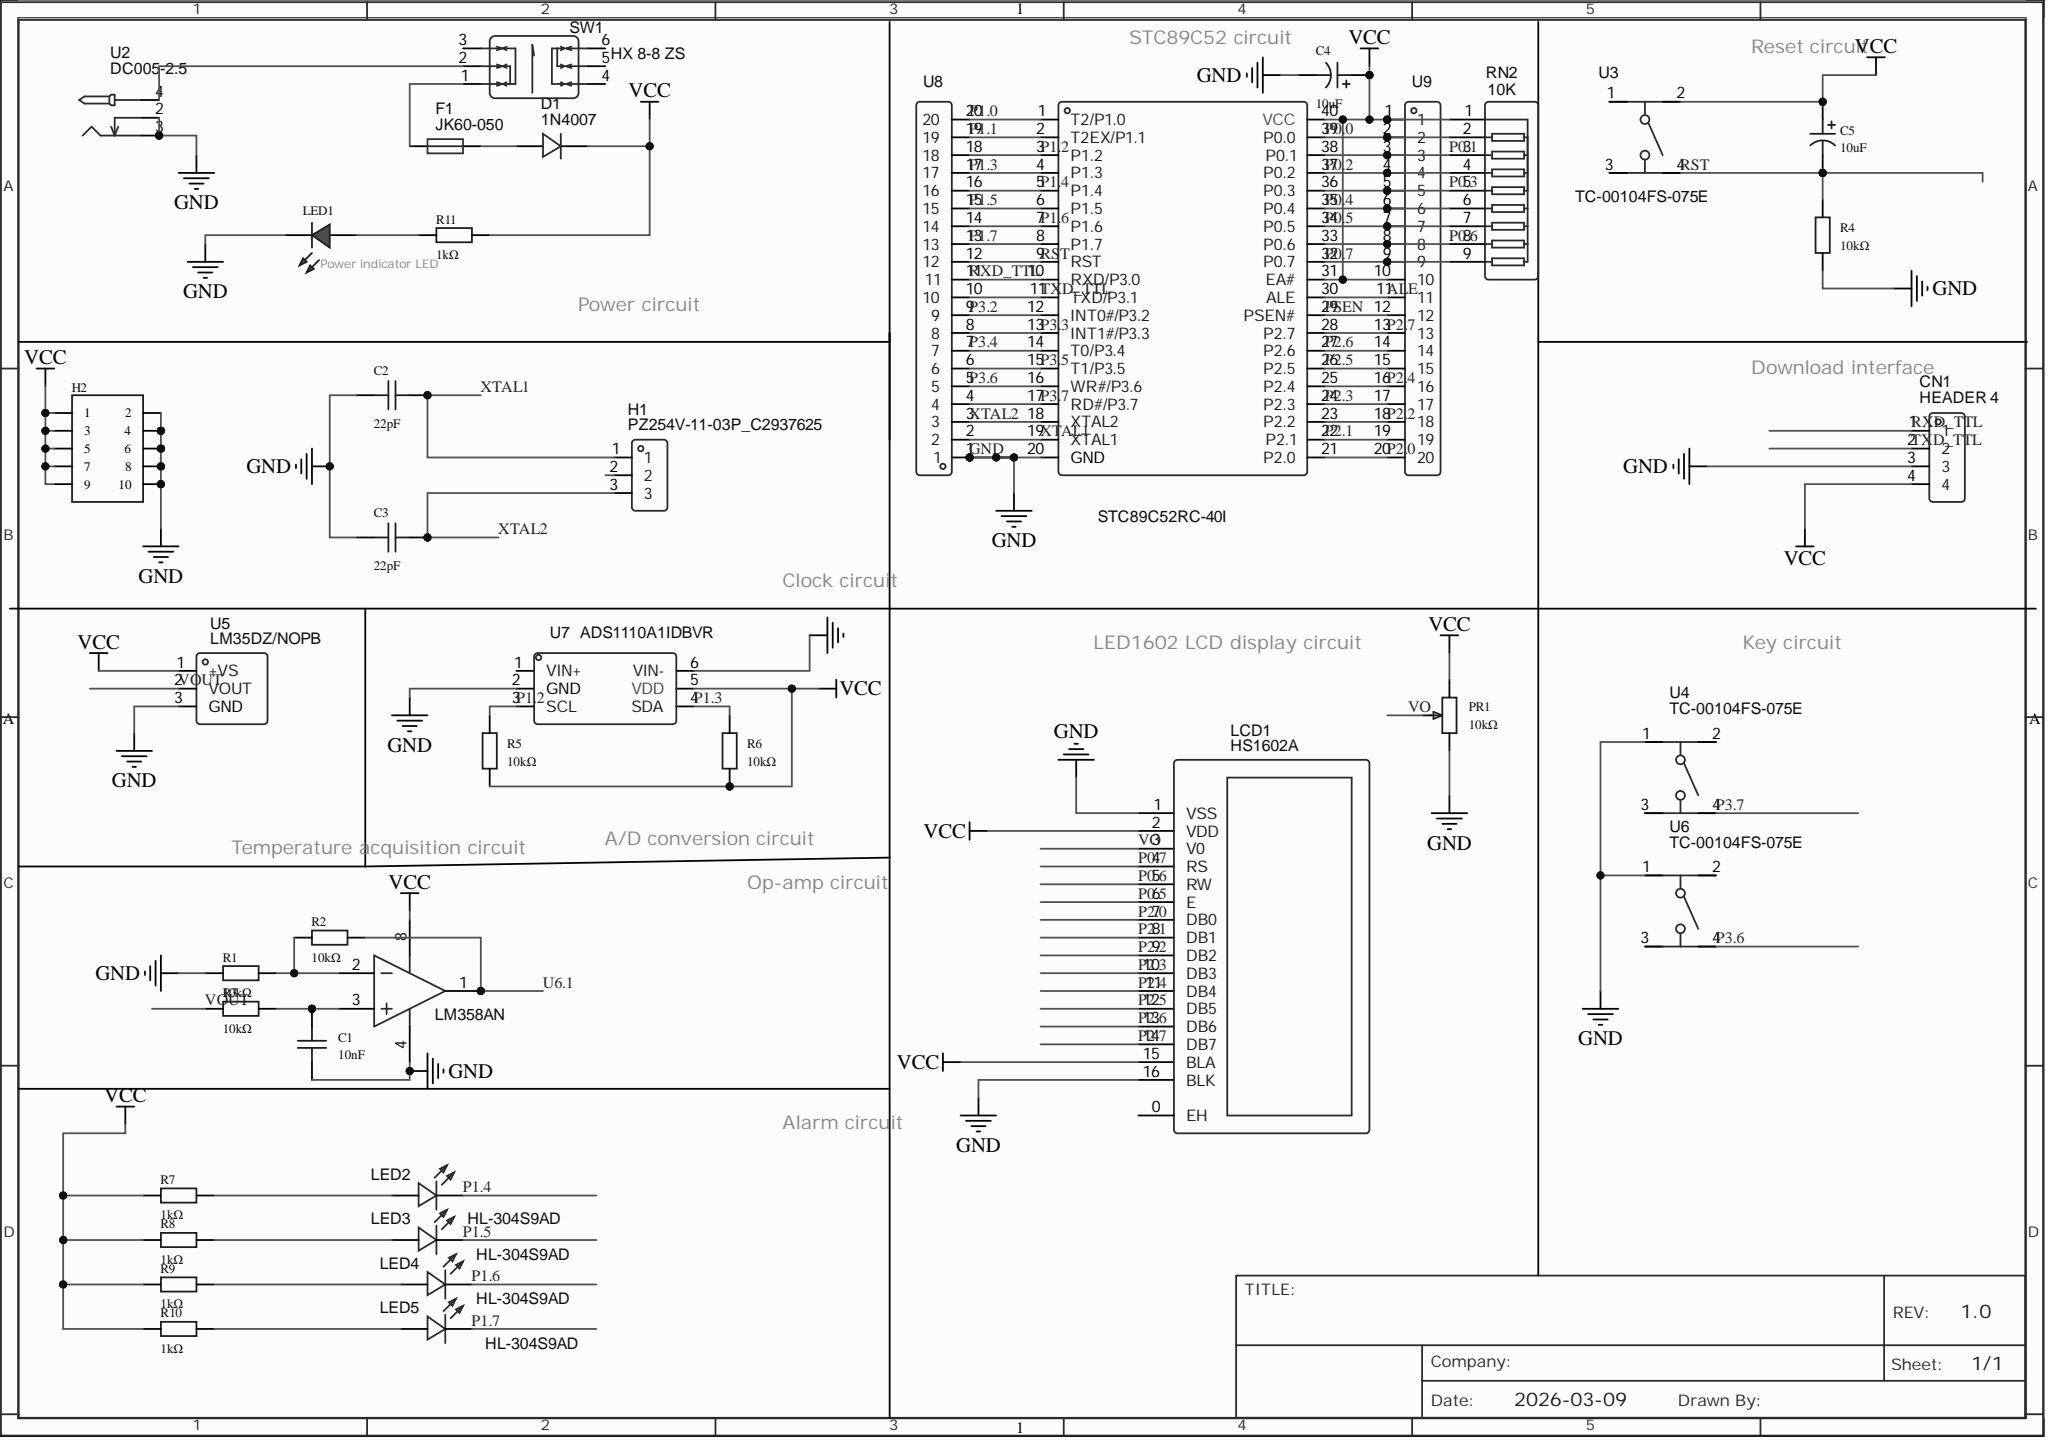Circuit board | Altium Designer | 40 parts | 52 nets
Bill of materials:
Comment,Description,Designator,Footprint,LibRef,Quantity
"10nF","容值:10nF;精度:±5%;额定电压:50V;温度系数:C0G；NP0;","C1","CAP-TH_L4.5-W2.5-P5.00-D0.5","FK24C0G1H103JN006","1"
"22pF","容值:22pF;精度:±5%;额定电压:50V;温度系数:-;","C2, C3","CAP-TH_L4.8-W3.2-P5.08-D0.5","CC4-0805-CG-50V-22pF-J","2"
"10uF","","C4, C5","CAP-TH_BD5.0-P2.00-D0.8-FD-10UF50VC110GL","10UF50VC110GL","2"
"HEADER 4","","CN1","CONN-TH_XH-4A","Header 4","1"
"1N4007","","D1","DO-41_BD2.4-L4.7-P8.70-D0.9-RD","1N4007","1"
"JK60-050","","F1","FUSE-TH_L8.9-W3.0-P5.10-D0.6-S1.20","JK60-050","1"
"PZ254V-11-03P_C2937625","","H1","HDR-TH_3P-P2.54-V-M_PZ254V-11-03P","PZ254V-11-03P","1"
"","","H2","HDR-TH_10P-P2.54-V-F-R2-C5-S2.54","HDR-F_2.54_2x5","1"
"HS1602A","","LCD1","LCD1602","HS1602A","1"
"","","LED1","LED_TH-3mm","LED_TH-R_3mm","1"
"HL-304S9AD","","LED2, LED3, LED4, LED5","LED-TH_BD3.0-P2.54-FD","HL-304S9AD","4"
"10kΩ","","PR1","R_3296","R_3296","1"
"10kΩ","","R1, R2, R3, R4, R5, R6","Res_1/8W","Res_AXIAL-1/8W","6"
"1kΩ","","R7, R8, R9, R10, R11","Res_1/8W","Res_AXIAL-1/8W","5"
"10K","","RN2","RES-ARRAY-TH_9P-P2.54-D1.0","排阻 10 K 5%","1"
"HX 8-8 ZS","","SW1","SW-TH_6P-L8.0-W8.0-P2.50-TL","HX 8-8 ZS","1"
"LM358AN","","U1","DIP-8_L9.8-W6.6-P2.54-LS7.6-BL","LM358AN","1"
"DC005-2.5","","U2","DC-IN-TH_DC005-2.5MM","DC005-2.5","1"
"TC-00104FS-075E","","U3, U4, U6","KEY-TH_4P-L6.0-W6.0-P4.50-LS6.5","TC-00104FS-075E","3"
"LM35DZ/NOPB","","U5","TO-92-3_L4.8-W3.7-P2.54-L","LM35DZ/NOPB","1"
"ADS1110A1IDBVR","","U7","SOT-23-6_L2.9-W1.6-P0.95-LS2.8-BR","ADS1110A1IDBVR","1"
"[Plugin] 2.54MM 1*20P straight female header-H5.0","","U8, U9","HDR-TH_20P-P2.54_C9900009338","[插件] 2.54mm 1*20P 直排母-H5.0","2"
"STC89C52RC-40I","","U100","DIP-40_L52.0-W13.7-P2.54-LS15.2-BL","STC89C52RC-40I-PDIP40","1"
Netlist (Protel format):
[
C1
CAP-TH_L4.5-W2.5-P5.00-D0.5
10nF



]
[
C2
CAP-TH_L4.8-W3.2-P5.08-D0.5
22pF



]
[
C3
CAP-TH_L4.8-W3.2-P5.08-D0.5
22pF



]
[
C4
CAP-TH_BD5.0-P2.00-D0.8-FD-10UF50VC110GL
10uF



]
[
C5
CAP-TH_BD5.0-P2.00-D0.8-FD-10UF50VC110GL
10uF



]
[
CN1
CONN-TH_XH-4A
HEADER 4



]
[
D1
DO-41_BD2.4-L4.7-P8.70-D0.9-RD
1N4007



]
[
F1
FUSE-TH_L8.9-W3.0-P5.10-D0.6-S1.20
JK60-050



]
[
H1
HDR-TH_3P-P2.54-V-M_PZ254V-11-03P
PZ254V-11-03P_C2937625



]
[
H2
HDR-TH_10P-P2.54-V-F-R2-C5-S2.54




]
[
LCD1
LCD1602
HS1602A



]
[
LED1
LED_TH-3mm




]
[
LED2
LED-TH_BD3.0-P2.54-FD
HL-304S9AD



]
[
LED3
LED-TH_BD3.0-P2.54-FD
HL-304S9AD



]
[
LED4
LED-TH_BD3.0-P2.54-FD
HL-304S9AD



]
[
LED5
LED-TH_BD3.0-P2.54-FD
HL-304S9AD



]
[
PR1
R_3296
10kΩ



]
[
R1
Res_1/8W
10kΩ



]
[
R2
Res_1/8W
10kΩ



]
[
R3
Res_1/8W
10kΩ



]
[
R4
Res_1/8W
10kΩ



]
[
R5
Res_1/8W
10kΩ



]
[
R6
Res_1/8W
10kΩ



]
[
R7
Res_1/8W
1kΩ



]
[
R8
Res_1/8W
1kΩ



]
[
R9
Res_1/8W
1kΩ



]
[
R10
Res_1/8W
1kΩ



]
[
R11
Res_1/8W
1kΩ



]
[
RN2
RES-ARRAY-TH_9P-P2.54-D1.0
10K



]
[
SW1
SW-TH_6P-L8.0-W8.0-P2.50-TL
HX 8-8 ZS



]
[
U1
DIP-8_L9.8-W6.6-P2.54-LS7.6-BL
LM358AN



]
[
U2
DC-IN-TH_DC005-2.5MM
DC005-2.5



]
[
U3
KEY-TH_4P-L6.0-W6.0-P4.50-LS6.5
TC-00104FS-075E



]
[
U4
KEY-TH_4P-L6.0-W6.0-P4.50-LS6.5
TC-00104FS-075E



]
[
U5
TO-92-3_L4.8-W3.7-P2.54-L
LM35DZ/NOPB



]
[
U6
KEY-TH_4P-L6.0-W6.0-P4.50-LS6.5
TC-00104FS-075E



]
[
U7
SOT-23-6_L2.9-W1.6-P0.95-LS2.8-BR
ADS1110A1IDBVR



]
[
U8
HDR-TH_20P-P2.54_C9900009338
[Plugin] 2.54MM 1*20P straight female header-H5.0



]
[
U9
HDR-TH_20P-P2.54_C9900009338
[Plugin] 2.54MM 1*20P straight female header-H5.0



]
[
U100
DIP-40_L52.0-W13.7-P2.54-LS15.2-BL
STC89C52RC-40I



]
(
XTAL2
C3-2
H1-3
U8-3
U100-18
)
(
XTAL1
C2-2
H1-1
U8-2
U100-19
)
(
VOUT
R3-1
U5-2
)
(
VO
LCD1-3
PR1-2
)
(
VCC
C4-1
C5-1
CN1-4
D1-1
H2-1
H2-3
H2-5
H2-7
H2-9
LCD1-2
LCD1-15
PR1-1
R5-1
R6-1
R7-1
R8-1
R9-1
R10-1
R11-2
RN2-1
U1-8
U3-2
U5-1
U7-5
U9-1
U9-10
U100-31
U100-40
)
(
U6.1
R2-2
U1-1
)
(
TXD_TTL
CN1-2
U8-10
U100-11
)
(
RXD_TTL
CN1-1
U8-11
U100-10
)
(
RST
C5-2
R4-2
U3-4
U8-12
U100-9
)
(
PSEN
U9-12
U100-29
)
(
P3.7
U4-4
U8-4
U100-17
)
(
P3.6
U6-4
U8-5
U100-16
)
(
P3.5
U8-6
U100-15
)
(
P3.4
U8-7
U100-14
)
(
P3.3
U8-8
U100-13
)
(
P3.2
U8-9
U100-12
)
(
P2.7
LCD1-14
U9-13
U100-28
)
(
P2.6
LCD1-13
U9-14
U100-27
)
(
P2.5
LCD1-12
U9-15
U100-26
)
(
P2.4
LCD1-11
U9-16
U100-25
)
(
P2.3
LCD1-10
U9-17
U100-24
)
(
P2.2
LCD1-9
U9-18
U100-23
)
(
P2.1
LCD1-8
U9-19
U100-22
)
(
P2.0
LCD1-7
U9-20
U100-21
)
(
P1.7
LED5-2
U8-13
U100-8
)
(
P1.6
LED4-2
U8-14
U100-7
)
(
P1.5
LED3-2
U8-15
U100-6
)
(
P1.4
LED2-2
U8-16
U100-5
)
(
P1.3
R6-2
U7-4
U8-17
U100-4
)
(
P1.2
R5-2
U7-3
U8-18
U100-3
)
(
P1.1
U8-19
U100-2
)
(
P1.0
U8-20
U100-1
)
(
P0.7
LCD1-4
RN2-9
U9-9
U100-32
)
(
P0.6
LCD1-5
RN2-8
U9-8
U100-33
)
(
P0.5
LCD1-6
RN2-7
U9-7
U100-34
)
(
P0.4
RN2-6
U9-6
U100-35
)
(
P0.3
RN2-5
U9-5
U100-36
)
(
P0.2
RN2-4
U9-4
U100-37
)
(
P0.1
RN2-3
U9-3
U100-38
)
(
P0.0
RN2-2
U9-2
U100-39
)
(
NetSW1_2
SW1-2
U2-4
)
(
NetR1_2
R1-2
R2-1
U1-2
)
(
NetLED5_1
LED5-1
R10-2
)
(
NetLED4_1
LED4-1
R9-2
)
(
NetLED3_1
LED3-1
R8-2
)
(
NetLED2_1
LED2-1
R7-2
)
(
NetLED1_1
LED1-1
R11-1
)
(
NetF1_1
F1-1
SW1-1
)
(
NetD1_2
D1-2
F1-2
)
(
NetC1_2
C1-2
R3-2
U1-3
)
(
GND
C1-1
C2-1
C3-1
C4-2
CN1-3
H2-2
H2-4
H2-6
H2-8
H2-10
LCD1-1
LCD1-16
LED1-2
PR1-3
R1-1
R4-1
U1-4
U2-2
U2-3
U4-1
U5-3
U6-1
U7-2
U7-6
U8-1
U100-20
)
(
ALE
U9-11
U100-30
)